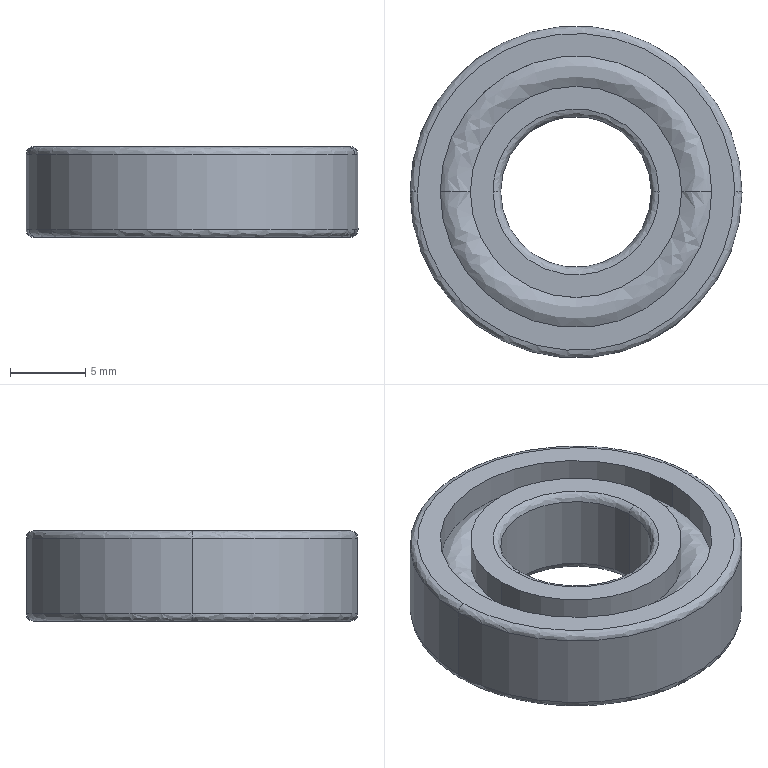Part | SolidWorks | features BaseBody 1 | 1 solid | 28 faces | box 22 x 22 x 6 mm | volume 1473 mm3 | spline 12 | cylinder 12 | plane 4 | commonest cylinder face diameters 14 x4 18 x4 10 x2 22 x2
STEP:
#1=CARTESIAN_POINT('',(11.,0.,2.5));
#2=VERTEX_POINT('',#1);
#3=CARTESIAN_POINT('',(-11.,0.,2.5));
#4=VERTEX_POINT('',#3);
#5=CARTESIAN_POINT('',(0.,0.,2.5));
#6=DIRECTION('',(0.,0.,-1.));
#7=DIRECTION('',(1.,0.,0.));
#8=AXIS2_PLACEMENT_3D('',#5,#6,#7);
#9=CIRCLE('',#8,11.);
#10=EDGE_CURVE('',#2,#4,#9,.T.);
#11=ORIENTED_EDGE('',*,*,#10,.F.);
#12=CARTESIAN_POINT('',(10.5,0.,3.));
#13=VERTEX_POINT('',#12);
#14=CARTESIAN_POINT('',(10.5,0.,2.5));
#15=DIRECTION('',(0.,-1.,0.));
#16=DIRECTION('',(1.,0.,0.));
#17=AXIS2_PLACEMENT_3D('',#14,#15,#16);
#18=CIRCLE('',#17,0.5);
#19=EDGE_CURVE('',#2,#13,#18,.T.);
#20=ORIENTED_EDGE('',*,*,#19,.T.);
#21=CARTESIAN_POINT('',(-10.5,0.,3.));
#22=VERTEX_POINT('',#21);
#23=CARTESIAN_POINT('',(10.5,0.,3.));
#24=CARTESIAN_POINT('',(10.5,-21.,3.));
#25=CARTESIAN_POINT('',(-10.5,-21.,3.));
#26=CARTESIAN_POINT('',(-10.5,0.,3.));
#27=(BOUNDED_CURVE()B_SPLINE_CURVE(3,(#23,#24,#25,#26),.UNSPECIFIED.,.F.,.T.)B_SPLINE_CURVE_WITH_KNOTS((4,4),(0.,1.),.UNSPECIFIED.)CURVE()GEOMETRIC_REPRESENTATION_ITEM()RATIONAL_B_SPLINE_CURVE((1.,0.3333,0.3333,1.))REPRESENTATION_ITEM(''));
#28=EDGE_CURVE('',#13,#22,#27,.T.);
#29=ORIENTED_EDGE('',*,*,#28,.T.);
#30=CARTESIAN_POINT('',(-10.5,0.,2.5));
#31=DIRECTION('',(0.,1.,0.));
#32=DIRECTION('',(-1.,0.,0.));
#33=AXIS2_PLACEMENT_3D('',#30,#31,#32);
#34=CIRCLE('',#33,0.5);
#35=EDGE_CURVE('',#4,#22,#34,.T.);
#36=ORIENTED_EDGE('',*,*,#35,.F.);
#37=EDGE_LOOP('',(#11,#20,#29,#36));
#38=FACE_OUTER_BOUND('',#37,.T.);
#39=CARTESIAN_POINT('',(11.,0.,2.5));
#40=CARTESIAN_POINT('',(11.,-22.,2.5));
#41=CARTESIAN_POINT('',(-11.,-22.,2.5));
#42=CARTESIAN_POINT('',(-11.,0.,2.5));
#43=CARTESIAN_POINT('',(11.,0.,2.793));
#44=CARTESIAN_POINT('',(11.,-22.,2.793));
#45=CARTESIAN_POINT('',(-11.,-22.,2.793));
#46=CARTESIAN_POINT('',(-11.,0.,2.793));
#47=CARTESIAN_POINT('',(10.793,0.,3.));
#48=CARTESIAN_POINT('',(10.793,-21.586,3.));
#49=CARTESIAN_POINT('',(-10.793,-21.586,3.));
#50=CARTESIAN_POINT('',(-10.793,0.,3.));
#51=CARTESIAN_POINT('',(10.5,0.,3.));
#52=CARTESIAN_POINT('',(10.5,-21.,3.));
#53=CARTESIAN_POINT('',(-10.5,-21.,3.));
#54=CARTESIAN_POINT('',(-10.5,0.,3.));
#55=(BOUNDED_SURFACE()B_SPLINE_SURFACE(3,3,((#39,#40,#41,#42),(#43,#44,#45,#46),(#47,#48,#49,#50),(#51,#52,#53,#54)),.UNSPECIFIED.,.F.,.F.,.T.)B_SPLINE_SURFACE_WITH_KNOTS((4,4),(4,4),(0.,1.),(0.,1.),.UNSPECIFIED.)GEOMETRIC_REPRESENTATION_ITEM()RATIONAL_B_SPLINE_SURFACE(((1.,0.3333,0.3333,1.),(0.8047,0.2682,0.2682,0.8047),(0.8047,0.2682,0.2682,0.8047),(1.,0.3333,0.3333,1.)))REPRESENTATION_ITEM('')SURFACE());
#56=ADVANCED_FACE('',(#38),#55,.T.);
#57=CARTESIAN_POINT('',(-11.,0.,-2.5));
#58=VERTEX_POINT('',#57);
#59=CARTESIAN_POINT('',(11.,0.,-2.5));
#60=VERTEX_POINT('',#59);
#61=CARTESIAN_POINT('',(0.,0.,-2.5));
#62=DIRECTION('',(0.,0.,1.));
#63=DIRECTION('',(1.,0.,0.));
#64=AXIS2_PLACEMENT_3D('',#61,#62,#63);
#65=CIRCLE('',#64,11.);
#66=EDGE_CURVE('',#58,#60,#65,.T.);
#67=ORIENTED_EDGE('',*,*,#66,.F.);
#68=CARTESIAN_POINT('',(-10.5,0.,-3.));
#69=VERTEX_POINT('',#68);
#70=CARTESIAN_POINT('',(-10.5,0.,-2.5));
#71=DIRECTION('',(0.,-1.,0.));
#72=DIRECTION('',(-1.,0.,0.));
#73=AXIS2_PLACEMENT_3D('',#70,#71,#72);
#74=CIRCLE('',#73,0.5);
#75=EDGE_CURVE('',#58,#69,#74,.T.);
#76=ORIENTED_EDGE('',*,*,#75,.T.);
#77=CARTESIAN_POINT('',(10.5,0.,-3.));
#78=VERTEX_POINT('',#77);
#79=CARTESIAN_POINT('',(-10.5,0.,-3.));
#80=CARTESIAN_POINT('',(-10.5,-21.,-3.));
#81=CARTESIAN_POINT('',(10.5,-21.,-3.));
#82=CARTESIAN_POINT('',(10.5,0.,-3.));
#83=(BOUNDED_CURVE()B_SPLINE_CURVE(3,(#79,#80,#81,#82),.UNSPECIFIED.,.F.,.T.)B_SPLINE_CURVE_WITH_KNOTS((4,4),(0.,1.),.UNSPECIFIED.)CURVE()GEOMETRIC_REPRESENTATION_ITEM()RATIONAL_B_SPLINE_CURVE((1.,0.3333,0.3333,1.))REPRESENTATION_ITEM(''));
#84=EDGE_CURVE('',#69,#78,#83,.T.);
#85=ORIENTED_EDGE('',*,*,#84,.T.);
#86=CARTESIAN_POINT('',(10.5,0.,-2.5));
#87=DIRECTION('',(0.,1.,0.));
#88=DIRECTION('',(1.,0.,0.));
#89=AXIS2_PLACEMENT_3D('',#86,#87,#88);
#90=CIRCLE('',#89,0.5);
#91=EDGE_CURVE('',#60,#78,#90,.T.);
#92=ORIENTED_EDGE('',*,*,#91,.F.);
#93=EDGE_LOOP('',(#67,#76,#85,#92));
#94=FACE_OUTER_BOUND('',#93,.T.);
#95=CARTESIAN_POINT('',(-11.,0.,-2.5));
#96=CARTESIAN_POINT('',(-11.,-22.,-2.5));
#97=CARTESIAN_POINT('',(11.,-22.,-2.5));
#98=CARTESIAN_POINT('',(11.,0.,-2.5));
#99=CARTESIAN_POINT('',(-11.,0.,-2.793));
#100=CARTESIAN_POINT('',(-11.,-22.,-2.793));
#101=CARTESIAN_POINT('',(11.,-22.,-2.793));
#102=CARTESIAN_POINT('',(11.,0.,-2.793));
#103=CARTESIAN_POINT('',(-10.793,0.,-3.));
#104=CARTESIAN_POINT('',(-10.793,-21.586,-3.));
#105=CARTESIAN_POINT('',(10.793,-21.586,-3.));
#106=CARTESIAN_POINT('',(10.793,0.,-3.));
#107=CARTESIAN_POINT('',(-10.5,0.,-3.));
#108=CARTESIAN_POINT('',(-10.5,-21.,-3.));
#109=CARTESIAN_POINT('',(10.5,-21.,-3.));
#110=CARTESIAN_POINT('',(10.5,0.,-3.));
#111=(BOUNDED_SURFACE()B_SPLINE_SURFACE(3,3,((#95,#96,#97,#98),(#99,#100,#101,#102),(#103,#104,#105,#106),(#107,#108,#109,#110)),.UNSPECIFIED.,.F.,.F.,.T.)B_SPLINE_SURFACE_WITH_KNOTS((4,4),(4,4),(0.,1.),(0.,1.),.UNSPECIFIED.)GEOMETRIC_REPRESENTATION_ITEM()RATIONAL_B_SPLINE_SURFACE(((1.,0.3333,0.3333,1.),(0.8047,0.2682,0.2682,0.8047),(0.8047,0.2682,0.2682,0.8047),(1.,0.3333,0.3333,1.)))REPRESENTATION_ITEM('')SURFACE());
#112=ADVANCED_FACE('',(#94),#111,.T.);
#113=CARTESIAN_POINT('',(-9.,0.,1.118));
#114=VERTEX_POINT('',#113);
#115=CARTESIAN_POINT('',(9.,0.,1.118));
#116=VERTEX_POINT('',#115);
#117=CARTESIAN_POINT('',(0.,0.,1.118));
#118=DIRECTION('',(0.,0.,1.));
#119=DIRECTION('',(1.,0.,0.));
#120=AXIS2_PLACEMENT_3D('',#117,#118,#119);
#121=CIRCLE('',#120,9.);
#122=EDGE_CURVE('',#114,#116,#121,.T.);
#123=ORIENTED_EDGE('',*,*,#122,.T.);
#124=CARTESIAN_POINT('',(7.,0.,1.118));
#125=VERTEX_POINT('',#124);
#126=CARTESIAN_POINT('',(8.,0.,0.));
#127=DIRECTION('',(0.,-1.,0.));
#128=DIRECTION('',(1.,0.,0.));
#129=AXIS2_PLACEMENT_3D('',#126,#127,#128);
#130=CIRCLE('',#129,1.5);
#131=EDGE_CURVE('',#116,#125,#130,.T.);
#132=ORIENTED_EDGE('',*,*,#131,.T.);
#133=CARTESIAN_POINT('',(-7.,0.,1.118));
#134=VERTEX_POINT('',#133);
#135=CARTESIAN_POINT('',(0.,0.,1.118));
#136=DIRECTION('',(0.,0.,-1.));
#137=DIRECTION('',(-1.,0.,0.));
#138=AXIS2_PLACEMENT_3D('',#135,#136,#137);
#139=CIRCLE('',#138,7.);
#140=EDGE_CURVE('',#125,#134,#139,.T.);
#141=ORIENTED_EDGE('',*,*,#140,.T.);
#142=CARTESIAN_POINT('',(-8.,0.,0.));
#143=DIRECTION('',(0.,1.,0.));
#144=DIRECTION('',(-1.,0.,0.));
#145=AXIS2_PLACEMENT_3D('',#142,#143,#144);
#146=CIRCLE('',#145,1.5);
#147=EDGE_CURVE('',#114,#134,#146,.T.);
#148=ORIENTED_EDGE('',*,*,#147,.F.);
#149=EDGE_LOOP('',(#123,#132,#141,#148));
#150=FACE_OUTER_BOUND('',#149,.T.);
#151=CARTESIAN_POINT('',(9.,0.,1.118));
#152=CARTESIAN_POINT('',(9.,-18.,1.118));
#153=CARTESIAN_POINT('',(-9.,-18.,1.118));
#154=CARTESIAN_POINT('',(-9.,0.,1.118));
#155=CARTESIAN_POINT('',(8.401,0.,1.653));
#156=CARTESIAN_POINT('',(8.401,-16.803,1.653));
#157=CARTESIAN_POINT('',(-8.401,-16.803,1.653));
#158=CARTESIAN_POINT('',(-8.401,0.,1.653));
#159=CARTESIAN_POINT('',(7.599,0.,1.653));
#160=CARTESIAN_POINT('',(7.599,-15.197,1.653));
#161=CARTESIAN_POINT('',(-7.599,-15.197,1.653));
#162=CARTESIAN_POINT('',(-7.599,0.,1.653));
#163=CARTESIAN_POINT('',(7.,0.,1.118));
#164=CARTESIAN_POINT('',(7.,-14.,1.118));
#165=CARTESIAN_POINT('',(-7.,-14.,1.118));
#166=CARTESIAN_POINT('',(-7.,0.,1.118));
#167=(BOUNDED_SURFACE()B_SPLINE_SURFACE(3,3,((#151,#152,#153,#154),(#155,#156,#157,#158),(#159,#160,#161,#162),(#163,#164,#165,#166)),.UNSPECIFIED.,.F.,.F.,.T.)B_SPLINE_SURFACE_WITH_KNOTS((4,4),(4,4),(0.,1.),(0.,1.),.UNSPECIFIED.)GEOMETRIC_REPRESENTATION_ITEM()RATIONAL_B_SPLINE_SURFACE(((1.,0.3333,0.3333,1.),(0.8302,0.2767,0.2767,0.8302),(0.8302,0.2767,0.2767,0.8302),(1.,0.3333,0.3333,1.)))REPRESENTATION_ITEM('')SURFACE());
#168=ADVANCED_FACE('',(#150),#167,.T.);
#169=CARTESIAN_POINT('',(-7.,0.,-1.118));
#170=VERTEX_POINT('',#169);
#171=CARTESIAN_POINT('',(7.,0.,-1.118));
#172=VERTEX_POINT('',#171);
#173=CARTESIAN_POINT('',(0.,0.,-1.118));
#174=DIRECTION('',(0.,0.,1.));
#175=DIRECTION('',(-1.,0.,0.));
#176=AXIS2_PLACEMENT_3D('',#173,#174,#175);
#177=CIRCLE('',#176,7.);
#178=EDGE_CURVE('',#170,#172,#177,.T.);
#179=ORIENTED_EDGE('',*,*,#178,.T.);
#180=CARTESIAN_POINT('',(9.,0.,-1.118));
#181=VERTEX_POINT('',#180);
#182=CARTESIAN_POINT('',(8.,0.,0.));
#183=DIRECTION('',(0.,-1.,0.));
#184=DIRECTION('',(1.,0.,0.));
#185=AXIS2_PLACEMENT_3D('',#182,#183,#184);
#186=CIRCLE('',#185,1.5);
#187=EDGE_CURVE('',#172,#181,#186,.T.);
#188=ORIENTED_EDGE('',*,*,#187,.T.);
#189=CARTESIAN_POINT('',(-9.,0.,-1.118));
#190=VERTEX_POINT('',#189);
#191=CARTESIAN_POINT('',(0.,0.,-1.118));
#192=DIRECTION('',(0.,0.,-1.));
#193=DIRECTION('',(1.,0.,0.));
#194=AXIS2_PLACEMENT_3D('',#191,#192,#193);
#195=CIRCLE('',#194,9.);
#196=EDGE_CURVE('',#181,#190,#195,.T.);
#197=ORIENTED_EDGE('',*,*,#196,.T.);
#198=CARTESIAN_POINT('',(-8.,0.,0.));
#199=DIRECTION('',(0.,1.,0.));
#200=DIRECTION('',(-1.,0.,0.));
#201=AXIS2_PLACEMENT_3D('',#198,#199,#200);
#202=CIRCLE('',#201,1.5);
#203=EDGE_CURVE('',#170,#190,#202,.T.);
#204=ORIENTED_EDGE('',*,*,#203,.F.);
#205=EDGE_LOOP('',(#179,#188,#197,#204));
#206=FACE_OUTER_BOUND('',#205,.T.);
#207=CARTESIAN_POINT('',(7.,0.,-1.118));
#208=CARTESIAN_POINT('',(7.,-14.,-1.118));
#209=CARTESIAN_POINT('',(-7.,-14.,-1.118));
#210=CARTESIAN_POINT('',(-7.,0.,-1.118));
#211=CARTESIAN_POINT('',(7.599,0.,-1.653));
#212=CARTESIAN_POINT('',(7.599,-15.197,-1.653));
#213=CARTESIAN_POINT('',(-7.599,-15.197,-1.653));
#214=CARTESIAN_POINT('',(-7.599,0.,-1.653));
#215=CARTESIAN_POINT('',(8.401,0.,-1.653));
#216=CARTESIAN_POINT('',(8.401,-16.803,-1.653));
#217=CARTESIAN_POINT('',(-8.401,-16.803,-1.653));
#218=CARTESIAN_POINT('',(-8.401,0.,-1.653));
#219=CARTESIAN_POINT('',(9.,0.,-1.118));
#220=CARTESIAN_POINT('',(9.,-18.,-1.118));
#221=CARTESIAN_POINT('',(-9.,-18.,-1.118));
#222=CARTESIAN_POINT('',(-9.,0.,-1.118));
#223=(BOUNDED_SURFACE()B_SPLINE_SURFACE(3,3,((#207,#208,#209,#210),(#211,#212,#213,#214),(#215,#216,#217,#218),(#219,#220,#221,#222)),.UNSPECIFIED.,.F.,.F.,.T.)B_SPLINE_SURFACE_WITH_KNOTS((4,4),(4,4),(0.,1.),(0.,1.),.UNSPECIFIED.)GEOMETRIC_REPRESENTATION_ITEM()RATIONAL_B_SPLINE_SURFACE(((1.,0.3333,0.3333,1.),(0.8302,0.2767,0.2767,0.8302),(0.8302,0.2767,0.2767,0.8302),(1.,0.3333,0.3333,1.)))REPRESENTATION_ITEM('')SURFACE());
#224=ADVANCED_FACE('',(#206),#223,.T.);
#225=CARTESIAN_POINT('',(-5.5,0.,3.));
#226=VERTEX_POINT('',#225);
#227=CARTESIAN_POINT('',(5.5,0.,3.));
#228=VERTEX_POINT('',#227);
#229=CARTESIAN_POINT('',(-5.5,0.,3.));
#230=CARTESIAN_POINT('',(-5.5,-11.,3.));
#231=CARTESIAN_POINT('',(5.5,-11.,3.));
#232=CARTESIAN_POINT('',(5.5,0.,3.));
#233=(BOUNDED_CURVE()B_SPLINE_CURVE(3,(#229,#230,#231,#232),.UNSPECIFIED.,.F.,.F.)B_SPLINE_CURVE_WITH_KNOTS((4,4),(0.,1.),.UNSPECIFIED.)CURVE()GEOMETRIC_REPRESENTATION_ITEM()RATIONAL_B_SPLINE_CURVE((1.,0.3333,0.3333,1.))REPRESENTATION_ITEM(''));
#234=EDGE_CURVE('',#226,#228,#233,.T.);
#235=ORIENTED_EDGE('',*,*,#234,.T.);
#236=CARTESIAN_POINT('',(5.,0.,2.5));
#237=VERTEX_POINT('',#236);
#238=CARTESIAN_POINT('',(5.5,0.,2.5));
#239=DIRECTION('',(0.,-1.,0.));
#240=DIRECTION('',(1.,0.,0.));
#241=AXIS2_PLACEMENT_3D('',#238,#239,#240);
#242=CIRCLE('',#241,0.5);
#243=EDGE_CURVE('',#228,#237,#242,.T.);
#244=ORIENTED_EDGE('',*,*,#243,.T.);
#245=CARTESIAN_POINT('',(-5.,0.,2.5));
#246=VERTEX_POINT('',#245);
#247=CARTESIAN_POINT('',(0.,0.,2.5));
#248=DIRECTION('',(0.,0.,-1.));
#249=DIRECTION('',(-1.,0.,0.));
#250=AXIS2_PLACEMENT_3D('',#247,#248,#249);
#251=CIRCLE('',#250,5.);
#252=EDGE_CURVE('',#237,#246,#251,.T.);
#253=ORIENTED_EDGE('',*,*,#252,.T.);
#254=CARTESIAN_POINT('',(-5.5,0.,2.5));
#255=DIRECTION('',(0.,1.,0.));
#256=DIRECTION('',(-1.,0.,0.));
#257=AXIS2_PLACEMENT_3D('',#254,#255,#256);
#258=CIRCLE('',#257,0.5);
#259=EDGE_CURVE('',#226,#246,#258,.T.);
#260=ORIENTED_EDGE('',*,*,#259,.F.);
#261=EDGE_LOOP('',(#235,#244,#253,#260));
#262=FACE_OUTER_BOUND('',#261,.T.);
#263=CARTESIAN_POINT('',(5.5,0.,3.));
#264=CARTESIAN_POINT('',(5.5,-11.,3.));
#265=CARTESIAN_POINT('',(-5.5,-11.,3.));
#266=CARTESIAN_POINT('',(-5.5,0.,3.));
#267=CARTESIAN_POINT('',(5.207,0.,3.));
#268=CARTESIAN_POINT('',(5.207,-10.414,3.));
#269=CARTESIAN_POINT('',(-5.207,-10.414,3.));
#270=CARTESIAN_POINT('',(-5.207,0.,3.));
#271=CARTESIAN_POINT('',(5.,0.,2.793));
#272=CARTESIAN_POINT('',(5.,-10.,2.793));
#273=CARTESIAN_POINT('',(-5.,-10.,2.793));
#274=CARTESIAN_POINT('',(-5.,0.,2.793));
#275=CARTESIAN_POINT('',(5.,0.,2.5));
#276=CARTESIAN_POINT('',(5.,-10.,2.5));
#277=CARTESIAN_POINT('',(-5.,-10.,2.5));
#278=CARTESIAN_POINT('',(-5.,0.,2.5));
#279=(BOUNDED_SURFACE()B_SPLINE_SURFACE(3,3,((#263,#264,#265,#266),(#267,#268,#269,#270),(#271,#272,#273,#274),(#275,#276,#277,#278)),.UNSPECIFIED.,.F.,.F.,.T.)B_SPLINE_SURFACE_WITH_KNOTS((4,4),(4,4),(0.,1.),(0.,1.),.UNSPECIFIED.)GEOMETRIC_REPRESENTATION_ITEM()RATIONAL_B_SPLINE_SURFACE(((1.,0.3333,0.3333,1.),(0.8047,0.2682,0.2682,0.8047),(0.8047,0.2682,0.2682,0.8047),(1.,0.3333,0.3333,1.)))REPRESENTATION_ITEM('')SURFACE());
#280=ADVANCED_FACE('',(#262),#279,.T.);
#281=CARTESIAN_POINT('',(5.5,0.,-3.));
#282=VERTEX_POINT('',#281);
#283=CARTESIAN_POINT('',(-5.5,0.,-3.));
#284=VERTEX_POINT('',#283);
#285=CARTESIAN_POINT('',(5.5,0.,-3.));
#286=CARTESIAN_POINT('',(5.5,-11.,-3.));
#287=CARTESIAN_POINT('',(-5.5,-11.,-3.));
#288=CARTESIAN_POINT('',(-5.5,0.,-3.));
#289=(BOUNDED_CURVE()B_SPLINE_CURVE(3,(#285,#286,#287,#288),.UNSPECIFIED.,.F.,.F.)B_SPLINE_CURVE_WITH_KNOTS((4,4),(0.,1.),.UNSPECIFIED.)CURVE()GEOMETRIC_REPRESENTATION_ITEM()RATIONAL_B_SPLINE_CURVE((1.,0.3333,0.3333,1.))REPRESENTATION_ITEM(''));
#290=EDGE_CURVE('',#282,#284,#289,.T.);
#291=ORIENTED_EDGE('',*,*,#290,.T.);
#292=CARTESIAN_POINT('',(-5.,0.,-2.5));
#293=VERTEX_POINT('',#292);
#294=CARTESIAN_POINT('',(-5.5,0.,-2.5));
#295=DIRECTION('',(0.,-1.,0.));
#296=DIRECTION('',(-1.,0.,0.));
#297=AXIS2_PLACEMENT_3D('',#294,#295,#296);
#298=CIRCLE('',#297,0.5);
#299=EDGE_CURVE('',#284,#293,#298,.T.);
#300=ORIENTED_EDGE('',*,*,#299,.T.);
#301=CARTESIAN_POINT('',(5.,0.,-2.5));
#302=VERTEX_POINT('',#301);
#303=CARTESIAN_POINT('',(0.,0.,-2.5));
#304=DIRECTION('',(0.,0.,1.));
#305=DIRECTION('',(1.,0.,0.));
#306=AXIS2_PLACEMENT_3D('',#303,#304,#305);
#307=CIRCLE('',#306,5.);
#308=EDGE_CURVE('',#293,#302,#307,.T.);
#309=ORIENTED_EDGE('',*,*,#308,.T.);
#310=CARTESIAN_POINT('',(5.5,0.,-2.5));
#311=DIRECTION('',(0.,1.,0.));
#312=DIRECTION('',(1.,0.,0.));
#313=AXIS2_PLACEMENT_3D('',#310,#311,#312);
#314=CIRCLE('',#313,0.5);
#315=EDGE_CURVE('',#282,#302,#314,.T.);
#316=ORIENTED_EDGE('',*,*,#315,.F.);
#317=EDGE_LOOP('',(#291,#300,#309,#316));
#318=FACE_OUTER_BOUND('',#317,.T.);
#319=CARTESIAN_POINT('',(-5.5,0.,-3.));
#320=CARTESIAN_POINT('',(-5.5,-11.,-3.));
#321=CARTESIAN_POINT('',(5.5,-11.,-3.));
#322=CARTESIAN_POINT('',(5.5,0.,-3.));
#323=CARTESIAN_POINT('',(-5.207,0.,-3.));
#324=CARTESIAN_POINT('',(-5.207,-10.414,-3.));
#325=CARTESIAN_POINT('',(5.207,-10.414,-3.));
#326=CARTESIAN_POINT('',(5.207,0.,-3.));
#327=CARTESIAN_POINT('',(-5.,0.,-2.793));
#328=CARTESIAN_POINT('',(-5.,-10.,-2.793));
#329=CARTESIAN_POINT('',(5.,-10.,-2.793));
#330=CARTESIAN_POINT('',(5.,0.,-2.793));
#331=CARTESIAN_POINT('',(-5.,0.,-2.5));
#332=CARTESIAN_POINT('',(-5.,-10.,-2.5));
#333=CARTESIAN_POINT('',(5.,-10.,-2.5));
#334=CARTESIAN_POINT('',(5.,0.,-2.5));
#335=(BOUNDED_SURFACE()B_SPLINE_SURFACE(3,3,((#319,#320,#321,#322),(#323,#324,#325,#326),(#327,#328,#329,#330),(#331,#332,#333,#334)),.UNSPECIFIED.,.F.,.F.,.T.)B_SPLINE_SURFACE_WITH_KNOTS((4,4),(4,4),(0.,1.),(0.,1.),.UNSPECIFIED.)GEOMETRIC_REPRESENTATION_ITEM()RATIONAL_B_SPLINE_SURFACE(((1.,0.3333,0.3333,1.),(0.8047,0.2682,0.2682,0.8047),(0.8047,0.2682,0.2682,0.8047),(1.,0.3333,0.3333,1.)))REPRESENTATION_ITEM('')SURFACE());
#336=ADVANCED_FACE('',(#318),#335,.T.);
#337=CARTESIAN_POINT('',(0.,0.,-2.5));
#338=DIRECTION('',(0.,0.,1.));
#339=DIRECTION('',(1.,0.,0.));
#340=AXIS2_PLACEMENT_3D('',#337,#338,#339);
#341=CIRCLE('',#340,11.);
#342=EDGE_CURVE('',#60,#58,#341,.T.);
#343=ORIENTED_EDGE('',*,*,#342,.T.);
#344=CARTESIAN_POINT('',(-11.,0.,50.392));
#345=DIRECTION('',(0.,0.,1.));
#346=VECTOR('',#345,1000.);
#347=LINE('',#344,#346);
#348=EDGE_CURVE('',#58,#4,#347,.T.);
#349=ORIENTED_EDGE('',*,*,#348,.T.);
#350=CARTESIAN_POINT('',(0.,0.,2.5));
#351=DIRECTION('',(0.,0.,-1.));
#352=DIRECTION('',(1.,0.,0.));
#353=AXIS2_PLACEMENT_3D('',#350,#351,#352);
#354=CIRCLE('',#353,11.);
#355=EDGE_CURVE('',#4,#2,#354,.T.);
#356=ORIENTED_EDGE('',*,*,#355,.T.);
#357=CARTESIAN_POINT('',(11.,0.,50.392));
#358=DIRECTION('',(0.,0.,1.));
#359=VECTOR('',#358,1000.);
#360=LINE('',#357,#359);
#361=EDGE_CURVE('',#60,#2,#360,.T.);
#362=ORIENTED_EDGE('',*,*,#361,.F.);
#363=EDGE_LOOP('',(#343,#349,#356,#362));
#364=FACE_OUTER_BOUND('',#363,.T.);
#365=CARTESIAN_POINT('',(0.,0.,50.392));
#366=DIRECTION('',(0.,0.,1.));
#367=DIRECTION('',(1.,0.,0.));
#368=AXIS2_PLACEMENT_3D('',#365,#366,#367);
#369=CYLINDRICAL_SURFACE('',#368,11.);
#370=ADVANCED_FACE('',(#364),#369,.T.);
#371=ORIENTED_EDGE('',*,*,#122,.F.);
#372=CARTESIAN_POINT('',(-9.,0.,3.));
#373=VERTEX_POINT('',#372);
#374=CARTESIAN_POINT('',(-9.,0.,50.392));
#375=DIRECTION('',(0.,0.,1.));
#376=VECTOR('',#375,1000.);
#377=LINE('',#374,#376);
#378=EDGE_CURVE('',#114,#373,#377,.T.);
#379=ORIENTED_EDGE('',*,*,#378,.T.);
#380=CARTESIAN_POINT('',(9.,0.,3.));
#381=VERTEX_POINT('',#380);
#382=CARTESIAN_POINT('',(0.,0.,3.));
#383=DIRECTION('',(0.,0.,1.));
#384=DIRECTION('',(1.,0.,0.));
#385=AXIS2_PLACEMENT_3D('',#382,#383,#384);
#386=CIRCLE('',#385,9.);
#387=EDGE_CURVE('',#373,#381,#386,.T.);
#388=ORIENTED_EDGE('',*,*,#387,.T.);
#389=CARTESIAN_POINT('',(9.,0.,50.392));
#390=DIRECTION('',(0.,0.,1.));
#391=VECTOR('',#390,1000.);
#392=LINE('',#389,#391);
#393=EDGE_CURVE('',#116,#381,#392,.T.);
#394=ORIENTED_EDGE('',*,*,#393,.F.);
#395=EDGE_LOOP('',(#371,#379,#388,#394));
#396=FACE_OUTER_BOUND('',#395,.T.);
#397=CARTESIAN_POINT('',(0.,0.,50.392));
#398=DIRECTION('',(0.,0.,1.));
#399=DIRECTION('',(1.,0.,0.));
#400=AXIS2_PLACEMENT_3D('',#397,#398,#399);
#401=CYLINDRICAL_SURFACE('',#400,9.);
#402=ADVANCED_FACE('',(#396),#401,.F.);
#403=CARTESIAN_POINT('',(9.,0.,-3.));
#404=VERTEX_POINT('',#403);
#405=CARTESIAN_POINT('',(-9.,0.,-3.));
#406=VERTEX_POINT('',#405);
#407=CARTESIAN_POINT('',(0.,0.,-3.));
#408=DIRECTION('',(0.,0.,-1.));
#409=DIRECTION('',(1.,0.,0.));
#410=AXIS2_PLACEMENT_3D('',#407,#408,#409);
#411=CIRCLE('',#410,9.);
#412=EDGE_CURVE('',#404,#406,#411,.T.);
#413=ORIENTED_EDGE('',*,*,#412,.T.);
#414=CARTESIAN_POINT('',(-9.,0.,50.392));
#415=DIRECTION('',(0.,0.,1.));
#416=VECTOR('',#415,1000.);
#417=LINE('',#414,#416);
#418=EDGE_CURVE('',#406,#190,#417,.T.);
#419=ORIENTED_EDGE('',*,*,#418,.T.);
#420=ORIENTED_EDGE('',*,*,#196,.F.);
#421=CARTESIAN_POINT('',(9.,0.,50.392));
#422=DIRECTION('',(0.,0.,1.));
#423=VECTOR('',#422,1000.);
#424=LINE('',#421,#423);
#425=EDGE_CURVE('',#404,#181,#424,.T.);
#426=ORIENTED_EDGE('',*,*,#425,.F.);
#427=EDGE_LOOP('',(#413,#419,#420,#426));
#428=FACE_OUTER_BOUND('',#427,.T.);
#429=CARTESIAN_POINT('',(0.,0.,50.392));
#430=DIRECTION('',(0.,0.,1.));
#431=DIRECTION('',(1.,0.,0.));
#432=AXIS2_PLACEMENT_3D('',#429,#430,#431);
#433=CYLINDRICAL_SURFACE('',#432,9.);
#434=ADVANCED_FACE('',(#428),#433,.F.);
#435=CARTESIAN_POINT('',(0.,0.,1.118));
#436=DIRECTION('',(0.,0.,-1.));
#437=DIRECTION('',(-1.,0.,0.));
#438=AXIS2_PLACEMENT_3D('',#435,#436,#437);
#439=CIRCLE('',#438,7.);
#440=EDGE_CURVE('',#134,#125,#439,.T.);
#441=ORIENTED_EDGE('',*,*,#440,.F.);
#442=CARTESIAN_POINT('',(-7.,0.,3.));
#443=VERTEX_POINT('',#442);
#444=CARTESIAN_POINT('',(-7.,0.,70.863));
#445=DIRECTION('',(0.,0.,1.));
#446=VECTOR('',#445,1000.);
#447=LINE('',#444,#446);
#448=EDGE_CURVE('',#134,#443,#447,.T.);
#449=ORIENTED_EDGE('',*,*,#448,.T.);
#450=CARTESIAN_POINT('',(7.,0.,3.));
#451=VERTEX_POINT('',#450);
#452=CARTESIAN_POINT('',(0.,0.,3.));
#453=DIRECTION('',(0.,0.,-1.));
#454=DIRECTION('',(1.,0.,0.));
#455=AXIS2_PLACEMENT_3D('',#452,#453,#454);
#456=CIRCLE('',#455,7.);
#457=EDGE_CURVE('',#443,#451,#456,.T.);
#458=ORIENTED_EDGE('',*,*,#457,.T.);
#459=CARTESIAN_POINT('',(7.,0.,70.863));
#460=DIRECTION('',(0.,0.,1.));
#461=VECTOR('',#460,1000.);
#462=LINE('',#459,#461);
#463=EDGE_CURVE('',#125,#451,#462,.T.);
#464=ORIENTED_EDGE('',*,*,#463,.F.);
#465=EDGE_LOOP('',(#441,#449,#458,#464));
#466=FACE_OUTER_BOUND('',#465,.T.);
#467=CARTESIAN_POINT('',(0.,0.,70.863));
#468=DIRECTION('',(0.,0.,1.));
#469=DIRECTION('',(1.,0.,0.));
#470=AXIS2_PLACEMENT_3D('',#467,#468,#469);
#471=CYLINDRICAL_SURFACE('',#470,7.);
#472=ADVANCED_FACE('',(#466),#471,.T.);
#473=CARTESIAN_POINT('',(7.,0.,-3.));
#474=VERTEX_POINT('',#473);
#475=CARTESIAN_POINT('',(-7.,0.,-3.));
#476=VERTEX_POINT('',#475);
#477=CARTESIAN_POINT('',(0.,0.,-3.));
#478=DIRECTION('',(0.,0.,1.));
#479=DIRECTION('',(1.,0.,0.));
#480=AXIS2_PLACEMENT_3D('',#477,#478,#479);
#481=CIRCLE('',#480,7.);
#482=EDGE_CURVE('',#474,#476,#481,.T.);
#483=ORIENTED_EDGE('',*,*,#482,.T.);
#484=CARTESIAN_POINT('',(-7.,0.,70.863));
#485=DIRECTION('',(0.,0.,1.));
#486=VECTOR('',#485,1000.);
#487=LINE('',#484,#486);
#488=EDGE_CURVE('',#476,#170,#487,.T.);
#489=ORIENTED_EDGE('',*,*,#488,.T.);
#490=CARTESIAN_POINT('',(0.,0.,-1.118));
#491=DIRECTION('',(0.,0.,1.));
#492=DIRECTION('',(-1.,0.,0.));
#493=AXIS2_PLACEMENT_3D('',#490,#491,#492);
#494=CIRCLE('',#493,7.);
#495=EDGE_CURVE('',#172,#170,#494,.T.);
#496=ORIENTED_EDGE('',*,*,#495,.F.);
#497=CARTESIAN_POINT('',(7.,0.,70.863));
#498=DIRECTION('',(0.,0.,1.));
#499=VECTOR('',#498,1000.);
#500=LINE('',#497,#499);
#501=EDGE_CURVE('',#474,#172,#500,.T.);
#502=ORIENTED_EDGE('',*,*,#501,.F.);
#503=EDGE_LOOP('',(#483,#489,#496,#502));
#504=FACE_OUTER_BOUND('',#503,.T.);
#505=CARTESIAN_POINT('',(0.,0.,70.863));
#506=DIRECTION('',(0.,0.,1.));
#507=DIRECTION('',(1.,0.,0.));
#508=AXIS2_PLACEMENT_3D('',#505,#506,#507);
#509=CYLINDRICAL_SURFACE('',#508,7.);
#510=ADVANCED_FACE('',(#504),#509,.T.);
#511=ORIENTED_EDGE('',*,*,#308,.F.);
#512=CARTESIAN_POINT('',(-5.,0.,70.863));
#513=DIRECTION('',(0.,0.,1.));
#514=VECTOR('',#513,1000.);
#515=LINE('',#512,#514);
#516=EDGE_CURVE('',#293,#246,#515,.T.);
#517=ORIENTED_EDGE('',*,*,#516,.T.);
#518=ORIENTED_EDGE('',*,*,#252,.F.);
#519=CARTESIAN_POINT('',(5.,0.,70.863));
#520=DIRECTION('',(0.,0.,1.));
#521=VECTOR('',#520,1000.);
#522=LINE('',#519,#521);
#523=EDGE_CURVE('',#302,#237,#522,.T.);
#524=ORIENTED_EDGE('',*,*,#523,.F.);
#525=EDGE_LOOP('',(#511,#517,#518,#524));
#526=FACE_OUTER_BOUND('',#525,.T.);
#527=CARTESIAN_POINT('',(0.,0.,70.863));
#528=DIRECTION('',(0.,0.,1.));
#529=DIRECTION('',(1.,0.,0.));
#530=AXIS2_PLACEMENT_3D('',#527,#528,#529);
#531=CYLINDRICAL_SURFACE('',#530,5.);
#532=ADVANCED_FACE('',(#526),#531,.F.);
#533=ORIENTED_EDGE('',*,*,#348,.F.);
#534=ORIENTED_EDGE('',*,*,#66,.T.);
#535=ORIENTED_EDGE('',*,*,#361,.T.);
#536=ORIENTED_EDGE('',*,*,#10,.T.);
#537=EDGE_LOOP('',(#533,#534,#535,#536));
#538=FACE_OUTER_BOUND('',#537,.T.);
#539=CARTESIAN_POINT('',(0.,0.,50.392));
#540=DIRECTION('',(0.,0.,1.));
#541=DIRECTION('',(1.,0.,0.));
#542=AXIS2_PLACEMENT_3D('',#539,#540,#541);
#543=CYLINDRICAL_SURFACE('',#542,11.);
#544=ADVANCED_FACE('',(#538),#543,.T.);
#545=ORIENTED_EDGE('',*,*,#19,.F.);
#546=ORIENTED_EDGE('',*,*,#355,.F.);
#547=ORIENTED_EDGE('',*,*,#35,.T.);
#548=CARTESIAN_POINT('',(-10.5,0.,3.));
#549=CARTESIAN_POINT('',(-10.5,21.,3.));
#550=CARTESIAN_POINT('',(10.5,21.,3.));
#551=CARTESIAN_POINT('',(10.5,0.,3.));
#552=(BOUNDED_CURVE()B_SPLINE_CURVE(3,(#548,#549,#550,#551),.UNSPECIFIED.,.F.,.T.)B_SPLINE_CURVE_WITH_KNOTS((4,4),(0.,1.),.UNSPECIFIED.)CURVE()GEOMETRIC_REPRESENTATION_ITEM()RATIONAL_B_SPLINE_CURVE((1.,0.3333,0.3333,1.))REPRESENTATION_ITEM(''));
#553=EDGE_CURVE('',#22,#13,#552,.T.);
#554=ORIENTED_EDGE('',*,*,#553,.T.);
#555=EDGE_LOOP('',(#545,#546,#547,#554));
#556=FACE_OUTER_BOUND('',#555,.T.);
#557=CARTESIAN_POINT('',(-11.,0.,2.5));
#558=CARTESIAN_POINT('',(-11.,22.,2.5));
#559=CARTESIAN_POINT('',(11.,22.,2.5));
#560=CARTESIAN_POINT('',(11.,0.,2.5));
#561=CARTESIAN_POINT('',(-11.,0.,2.793));
#562=CARTESIAN_POINT('',(-11.,22.,2.793));
#563=CARTESIAN_POINT('',(11.,22.,2.793));
#564=CARTESIAN_POINT('',(11.,0.,2.793));
#565=CARTESIAN_POINT('',(-10.793,0.,3.));
#566=CARTESIAN_POINT('',(-10.793,21.586,3.));
#567=CARTESIAN_POINT('',(10.793,21.586,3.));
#568=CARTESIAN_POINT('',(10.793,0.,3.));
#569=CARTESIAN_POINT('',(-10.5,0.,3.));
#570=CARTESIAN_POINT('',(-10.5,21.,3.));
#571=CARTESIAN_POINT('',(10.5,21.,3.));
#572=CARTESIAN_POINT('',(10.5,0.,3.));
#573=(BOUNDED_SURFACE()B_SPLINE_SURFACE(3,3,((#557,#558,#559,#560),(#561,#562,#563,#564),(#565,#566,#567,#568),(#569,#570,#571,#572)),.UNSPECIFIED.,.F.,.F.,.T.)B_SPLINE_SURFACE_WITH_KNOTS((4,4),(4,4),(0.,1.),(0.,1.),.UNSPECIFIED.)GEOMETRIC_REPRESENTATION_ITEM()RATIONAL_B_SPLINE_SURFACE(((1.,0.3333,0.3333,1.),(0.8047,0.2682,0.2682,0.8047),(0.8047,0.2682,0.2682,0.8047),(1.,0.3333,0.3333,1.)))REPRESENTATION_ITEM('')SURFACE());
#574=ADVANCED_FACE('',(#556),#573,.T.);
#575=ORIENTED_EDGE('',*,*,#75,.F.);
#576=ORIENTED_EDGE('',*,*,#342,.F.);
#577=ORIENTED_EDGE('',*,*,#91,.T.);
#578=CARTESIAN_POINT('',(10.5,0.,-3.));
#579=CARTESIAN_POINT('',(10.5,21.,-3.));
#580=CARTESIAN_POINT('',(-10.5,21.,-3.));
#581=CARTESIAN_POINT('',(-10.5,0.,-3.));
#582=(BOUNDED_CURVE()B_SPLINE_CURVE(3,(#578,#579,#580,#581),.UNSPECIFIED.,.F.,.T.)B_SPLINE_CURVE_WITH_KNOTS((4,4),(0.,1.),.UNSPECIFIED.)CURVE()GEOMETRIC_REPRESENTATION_ITEM()RATIONAL_B_SPLINE_CURVE((1.,0.3333,0.3333,1.))REPRESENTATION_ITEM(''));
#583=EDGE_CURVE('',#78,#69,#582,.T.);
#584=ORIENTED_EDGE('',*,*,#583,.T.);
#585=EDGE_LOOP('',(#575,#576,#577,#584));
#586=FACE_OUTER_BOUND('',#585,.T.);
#587=CARTESIAN_POINT('',(11.,0.,-2.5));
#588=CARTESIAN_POINT('',(11.,22.,-2.5));
#589=CARTESIAN_POINT('',(-11.,22.,-2.5));
#590=CARTESIAN_POINT('',(-11.,0.,-2.5));
#591=CARTESIAN_POINT('',(11.,0.,-2.793));
#592=CARTESIAN_POINT('',(11.,22.,-2.793));
#593=CARTESIAN_POINT('',(-11.,22.,-2.793));
#594=CARTESIAN_POINT('',(-11.,0.,-2.793));
#595=CARTESIAN_POINT('',(10.793,0.,-3.));
#596=CARTESIAN_POINT('',(10.793,21.586,-3.));
#597=CARTESIAN_POINT('',(-10.793,21.586,-3.));
#598=CARTESIAN_POINT('',(-10.793,0.,-3.));
#599=CARTESIAN_POINT('',(10.5,0.,-3.));
#600=CARTESIAN_POINT('',(10.5,21.,-3.));
#601=CARTESIAN_POINT('',(-10.5,21.,-3.));
#602=CARTESIAN_POINT('',(-10.5,0.,-3.));
#603=(BOUNDED_SURFACE()B_SPLINE_SURFACE(3,3,((#587,#588,#589,#590),(#591,#592,#593,#594),(#595,#596,#597,#598),(#599,#600,#601,#602)),.UNSPECIFIED.,.F.,.F.,.T.)B_SPLINE_SURFACE_WITH_KNOTS((4,4),(4,4),(0.,1.),(0.,1.),.UNSPECIFIED.)GEOMETRIC_REPRESENTATION_ITEM()RATIONAL_B_SPLINE_SURFACE(((1.,0.3333,0.3333,1.),(0.8047,0.2682,0.2682,0.8047),(0.8047,0.2682,0.2682,0.8047),(1.,0.3333,0.3333,1.)))REPRESENTATION_ITEM('')SURFACE());
#604=ADVANCED_FACE('',(#586),#603,.T.);
#605=CARTESIAN_POINT('',(0.,0.,3.));
#606=DIRECTION('',(0.,0.,1.));
#607=DIRECTION('',(1.,0.,0.));
#608=AXIS2_PLACEMENT_3D('',#605,#606,#607);
#609=CIRCLE('',#608,9.);
#610=EDGE_CURVE('',#381,#373,#609,.T.);
#611=ORIENTED_EDGE('',*,*,#610,.F.);
#612=ORIENTED_EDGE('',*,*,#387,.F.);
#613=EDGE_LOOP('',(#611,#612));
#614=FACE_BOUND('',#613,.T.);
#615=ORIENTED_EDGE('',*,*,#553,.F.);
#616=ORIENTED_EDGE('',*,*,#28,.F.);
#617=EDGE_LOOP('',(#615,#616));
#618=FACE_OUTER_BOUND('',#617,.T.);
#619=CARTESIAN_POINT('',(0.,11.,3.));
#620=DIRECTION('',(0.,0.,-1.));
#621=DIRECTION('',(-1.,0.,0.));
#622=AXIS2_PLACEMENT_3D('',#619,#620,#621);
#623=PLANE('',#622);
#624=ADVANCED_FACE('',(#614,#618),#623,.F.);
#625=ORIENTED_EDGE('',*,*,#412,.F.);
#626=CARTESIAN_POINT('',(0.,0.,-3.));
#627=DIRECTION('',(0.,0.,-1.));
#628=DIRECTION('',(1.,0.,0.));
#629=AXIS2_PLACEMENT_3D('',#626,#627,#628);
#630=CIRCLE('',#629,9.);
#631=EDGE_CURVE('',#406,#404,#630,.T.);
#632=ORIENTED_EDGE('',*,*,#631,.F.);
#633=EDGE_LOOP('',(#625,#632));
#634=FACE_BOUND('',#633,.T.);
#635=ORIENTED_EDGE('',*,*,#583,.F.);
#636=ORIENTED_EDGE('',*,*,#84,.F.);
#637=EDGE_LOOP('',(#635,#636));
#638=FACE_OUTER_BOUND('',#637,.T.);
#639=CARTESIAN_POINT('',(0.,11.,-3.));
#640=DIRECTION('',(0.,0.,1.));
#641=DIRECTION('',(1.,0.,0.));
#642=AXIS2_PLACEMENT_3D('',#639,#640,#641);
#643=PLANE('',#642);
#644=ADVANCED_FACE('',(#634,#638),#643,.F.);
#645=ORIENTED_EDGE('',*,*,#378,.F.);
#646=CARTESIAN_POINT('',(0.,0.,1.118));
#647=DIRECTION('',(0.,0.,1.));
#648=DIRECTION('',(1.,0.,0.));
#649=AXIS2_PLACEMENT_3D('',#646,#647,#648);
#650=CIRCLE('',#649,9.);
#651=EDGE_CURVE('',#116,#114,#650,.T.);
#652=ORIENTED_EDGE('',*,*,#651,.F.);
#653=ORIENTED_EDGE('',*,*,#393,.T.);
#654=ORIENTED_EDGE('',*,*,#610,.T.);
#655=EDGE_LOOP('',(#645,#652,#653,#654));
#656=FACE_OUTER_BOUND('',#655,.T.);
#657=CARTESIAN_POINT('',(0.,0.,50.392));
#658=DIRECTION('',(0.,0.,1.));
#659=DIRECTION('',(1.,0.,0.));
#660=AXIS2_PLACEMENT_3D('',#657,#658,#659);
#661=CYLINDRICAL_SURFACE('',#660,9.);
#662=ADVANCED_FACE('',(#656),#661,.F.);
#663=ORIENTED_EDGE('',*,*,#418,.F.);
#664=ORIENTED_EDGE('',*,*,#631,.T.);
#665=ORIENTED_EDGE('',*,*,#425,.T.);
#666=CARTESIAN_POINT('',(0.,0.,-1.118));
#667=DIRECTION('',(0.,0.,-1.));
#668=DIRECTION('',(1.,0.,0.));
#669=AXIS2_PLACEMENT_3D('',#666,#667,#668);
#670=CIRCLE('',#669,9.);
#671=EDGE_CURVE('',#190,#181,#670,.T.);
#672=ORIENTED_EDGE('',*,*,#671,.F.);
#673=EDGE_LOOP('',(#663,#664,#665,#672));
#674=FACE_OUTER_BOUND('',#673,.T.);
#675=CARTESIAN_POINT('',(0.,0.,50.392));
#676=DIRECTION('',(0.,0.,1.));
#677=DIRECTION('',(1.,0.,0.));
#678=AXIS2_PLACEMENT_3D('',#675,#676,#677);
#679=CYLINDRICAL_SURFACE('',#678,9.);
#680=ADVANCED_FACE('',(#674),#679,.F.);
#681=ORIENTED_EDGE('',*,*,#131,.F.);
#682=ORIENTED_EDGE('',*,*,#651,.T.);
#683=ORIENTED_EDGE('',*,*,#147,.T.);
#684=ORIENTED_EDGE('',*,*,#440,.T.);
#685=EDGE_LOOP('',(#681,#682,#683,#684));
#686=FACE_OUTER_BOUND('',#685,.T.);
#687=CARTESIAN_POINT('',(-9.,0.,1.118));
#688=CARTESIAN_POINT('',(-9.,18.,1.118));
#689=CARTESIAN_POINT('',(9.,18.,1.118));
#690=CARTESIAN_POINT('',(9.,0.,1.118));
#691=CARTESIAN_POINT('',(-8.401,0.,1.653));
#692=CARTESIAN_POINT('',(-8.401,16.803,1.653));
#693=CARTESIAN_POINT('',(8.401,16.803,1.653));
#694=CARTESIAN_POINT('',(8.401,0.,1.653));
#695=CARTESIAN_POINT('',(-7.599,0.,1.653));
#696=CARTESIAN_POINT('',(-7.599,15.197,1.653));
#697=CARTESIAN_POINT('',(7.599,15.197,1.653));
#698=CARTESIAN_POINT('',(7.599,0.,1.653));
#699=CARTESIAN_POINT('',(-7.,0.,1.118));
#700=CARTESIAN_POINT('',(-7.,14.,1.118));
#701=CARTESIAN_POINT('',(7.,14.,1.118));
#702=CARTESIAN_POINT('',(7.,0.,1.118));
#703=(BOUNDED_SURFACE()B_SPLINE_SURFACE(3,3,((#687,#688,#689,#690),(#691,#692,#693,#694),(#695,#696,#697,#698),(#699,#700,#701,#702)),.UNSPECIFIED.,.F.,.F.,.T.)B_SPLINE_SURFACE_WITH_KNOTS((4,4),(4,4),(0.,1.),(0.,1.),.UNSPECIFIED.)GEOMETRIC_REPRESENTATION_ITEM()RATIONAL_B_SPLINE_SURFACE(((1.,0.3333,0.3333,1.),(0.8302,0.2767,0.2767,0.8302),(0.8302,0.2767,0.2767,0.8302),(1.,0.3333,0.3333,1.)))REPRESENTATION_ITEM('')SURFACE());
#704=ADVANCED_FACE('',(#686),#703,.T.);
#705=ORIENTED_EDGE('',*,*,#187,.F.);
#706=ORIENTED_EDGE('',*,*,#495,.T.);
#707=ORIENTED_EDGE('',*,*,#203,.T.);
#708=ORIENTED_EDGE('',*,*,#671,.T.);
#709=EDGE_LOOP('',(#705,#706,#707,#708));
#710=FACE_OUTER_BOUND('',#709,.T.);
#711=CARTESIAN_POINT('',(-7.,0.,-1.118));
#712=CARTESIAN_POINT('',(-7.,14.,-1.118));
#713=CARTESIAN_POINT('',(7.,14.,-1.118));
#714=CARTESIAN_POINT('',(7.,0.,-1.118));
#715=CARTESIAN_POINT('',(-7.599,0.,-1.653));
#716=CARTESIAN_POINT('',(-7.599,15.197,-1.653));
#717=CARTESIAN_POINT('',(7.599,15.197,-1.653));
#718=CARTESIAN_POINT('',(7.599,0.,-1.653));
#719=CARTESIAN_POINT('',(-8.401,0.,-1.653));
#720=CARTESIAN_POINT('',(-8.401,16.803,-1.653));
#721=CARTESIAN_POINT('',(8.401,16.803,-1.653));
#722=CARTESIAN_POINT('',(8.401,0.,-1.653));
#723=CARTESIAN_POINT('',(-9.,0.,-1.118));
#724=CARTESIAN_POINT('',(-9.,18.,-1.118));
#725=CARTESIAN_POINT('',(9.,18.,-1.118));
#726=CARTESIAN_POINT('',(9.,0.,-1.118));
#727=(BOUNDED_SURFACE()B_SPLINE_SURFACE(3,3,((#711,#712,#713,#714),(#715,#716,#717,#718),(#719,#720,#721,#722),(#723,#724,#725,#726)),.UNSPECIFIED.,.F.,.F.,.T.)B_SPLINE_SURFACE_WITH_KNOTS((4,4),(4,4),(0.,1.),(0.,1.),.UNSPECIFIED.)GEOMETRIC_REPRESENTATION_ITEM()RATIONAL_B_SPLINE_SURFACE(((1.,0.3333,0.3333,1.),(0.8302,0.2767,0.2767,0.8302),(0.8302,0.2767,0.2767,0.8302),(1.,0.3333,0.3333,1.)))REPRESENTATION_ITEM('')SURFACE());
#728=ADVANCED_FACE('',(#710),#727,.T.);
#729=ORIENTED_EDGE('',*,*,#448,.F.);
#730=ORIENTED_EDGE('',*,*,#140,.F.);
#731=ORIENTED_EDGE('',*,*,#463,.T.);
#732=CARTESIAN_POINT('',(0.,0.,3.));
#733=DIRECTION('',(0.,0.,-1.));
#734=DIRECTION('',(1.,0.,0.));
#735=AXIS2_PLACEMENT_3D('',#732,#733,#734);
#736=CIRCLE('',#735,7.);
#737=EDGE_CURVE('',#451,#443,#736,.T.);
#738=ORIENTED_EDGE('',*,*,#737,.T.);
#739=EDGE_LOOP('',(#729,#730,#731,#738));
#740=FACE_OUTER_BOUND('',#739,.T.);
#741=CARTESIAN_POINT('',(0.,0.,70.863));
#742=DIRECTION('',(0.,0.,1.));
#743=DIRECTION('',(1.,0.,0.));
#744=AXIS2_PLACEMENT_3D('',#741,#742,#743);
#745=CYLINDRICAL_SURFACE('',#744,7.);
#746=ADVANCED_FACE('',(#740),#745,.T.);
#747=ORIENTED_EDGE('',*,*,#488,.F.);
#748=CARTESIAN_POINT('',(0.,0.,-3.));
#749=DIRECTION('',(0.,0.,1.));
#750=DIRECTION('',(1.,0.,0.));
#751=AXIS2_PLACEMENT_3D('',#748,#749,#750);
#752=CIRCLE('',#751,7.);
#753=EDGE_CURVE('',#476,#474,#752,.T.);
#754=ORIENTED_EDGE('',*,*,#753,.T.);
#755=ORIENTED_EDGE('',*,*,#501,.T.);
#756=ORIENTED_EDGE('',*,*,#178,.F.);
#757=EDGE_LOOP('',(#747,#754,#755,#756));
#758=FACE_OUTER_BOUND('',#757,.T.);
#759=CARTESIAN_POINT('',(0.,0.,70.863));
#760=DIRECTION('',(0.,0.,1.));
#761=DIRECTION('',(1.,0.,0.));
#762=AXIS2_PLACEMENT_3D('',#759,#760,#761);
#763=CYLINDRICAL_SURFACE('',#762,7.);
#764=ADVANCED_FACE('',(#758),#763,.T.);
#765=ORIENTED_EDGE('',*,*,#737,.F.);
#766=ORIENTED_EDGE('',*,*,#457,.F.);
#767=EDGE_LOOP('',(#765,#766));
#768=FACE_OUTER_BOUND('',#767,.T.);
#769=ORIENTED_EDGE('',*,*,#234,.F.);
#770=CARTESIAN_POINT('',(5.5,0.,3.));
#771=CARTESIAN_POINT('',(5.5,11.,3.));
#772=CARTESIAN_POINT('',(-5.5,11.,3.));
#773=CARTESIAN_POINT('',(-5.5,0.,3.));
#774=(BOUNDED_CURVE()B_SPLINE_CURVE(3,(#770,#771,#772,#773),.UNSPECIFIED.,.F.,.T.)B_SPLINE_CURVE_WITH_KNOTS((4,4),(0.,1.),.UNSPECIFIED.)CURVE()GEOMETRIC_REPRESENTATION_ITEM()RATIONAL_B_SPLINE_CURVE((1.,0.3333,0.3333,1.))REPRESENTATION_ITEM(''));
#775=EDGE_CURVE('',#228,#226,#774,.T.);
#776=ORIENTED_EDGE('',*,*,#775,.F.);
#777=EDGE_LOOP('',(#769,#776));
#778=FACE_BOUND('',#777,.T.);
#779=CARTESIAN_POINT('',(0.,5.,3.));
#780=DIRECTION('',(0.,0.,-1.));
#781=DIRECTION('',(-1.,0.,0.));
#782=AXIS2_PLACEMENT_3D('',#779,#780,#781);
#783=PLANE('',#782);
#784=ADVANCED_FACE('',(#768,#778),#783,.F.);
#785=ORIENTED_EDGE('',*,*,#482,.F.);
#786=ORIENTED_EDGE('',*,*,#753,.F.);
#787=EDGE_LOOP('',(#785,#786));
#788=FACE_OUTER_BOUND('',#787,.T.);
#789=ORIENTED_EDGE('',*,*,#290,.F.);
#790=CARTESIAN_POINT('',(-5.5,0.,-3.));
#791=CARTESIAN_POINT('',(-5.5,11.,-3.));
#792=CARTESIAN_POINT('',(5.5,11.,-3.));
#793=CARTESIAN_POINT('',(5.5,0.,-3.));
#794=(BOUNDED_CURVE()B_SPLINE_CURVE(3,(#790,#791,#792,#793),.UNSPECIFIED.,.F.,.T.)B_SPLINE_CURVE_WITH_KNOTS((4,4),(0.,1.),.UNSPECIFIED.)CURVE()GEOMETRIC_REPRESENTATION_ITEM()RATIONAL_B_SPLINE_CURVE((1.,0.3333,0.3333,1.))REPRESENTATION_ITEM(''));
#795=EDGE_CURVE('',#284,#282,#794,.T.);
#796=ORIENTED_EDGE('',*,*,#795,.F.);
#797=EDGE_LOOP('',(#789,#796));
#798=FACE_BOUND('',#797,.T.);
#799=CARTESIAN_POINT('',(0.,5.,-3.));
#800=DIRECTION('',(0.,0.,1.));
#801=DIRECTION('',(1.,0.,0.));
#802=AXIS2_PLACEMENT_3D('',#799,#800,#801);
#803=PLANE('',#802);
#804=ADVANCED_FACE('',(#788,#798),#803,.F.);
#805=ORIENTED_EDGE('',*,*,#243,.F.);
#806=ORIENTED_EDGE('',*,*,#775,.T.);
#807=ORIENTED_EDGE('',*,*,#259,.T.);
#808=CARTESIAN_POINT('',(0.,0.,2.5));
#809=DIRECTION('',(0.,0.,-1.));
#810=DIRECTION('',(-1.,0.,0.));
#811=AXIS2_PLACEMENT_3D('',#808,#809,#810);
#812=CIRCLE('',#811,5.);
#813=EDGE_CURVE('',#246,#237,#812,.T.);
#814=ORIENTED_EDGE('',*,*,#813,.T.);
#815=EDGE_LOOP('',(#805,#806,#807,#814));
#816=FACE_OUTER_BOUND('',#815,.T.);
#817=CARTESIAN_POINT('',(-5.5,0.,3.));
#818=CARTESIAN_POINT('',(-5.5,11.,3.));
#819=CARTESIAN_POINT('',(5.5,11.,3.));
#820=CARTESIAN_POINT('',(5.5,0.,3.));
#821=CARTESIAN_POINT('',(-5.207,0.,3.));
#822=CARTESIAN_POINT('',(-5.207,10.414,3.));
#823=CARTESIAN_POINT('',(5.207,10.414,3.));
#824=CARTESIAN_POINT('',(5.207,0.,3.));
#825=CARTESIAN_POINT('',(-5.,0.,2.793));
#826=CARTESIAN_POINT('',(-5.,10.,2.793));
#827=CARTESIAN_POINT('',(5.,10.,2.793));
#828=CARTESIAN_POINT('',(5.,0.,2.793));
#829=CARTESIAN_POINT('',(-5.,0.,2.5));
#830=CARTESIAN_POINT('',(-5.,10.,2.5));
#831=CARTESIAN_POINT('',(5.,10.,2.5));
#832=CARTESIAN_POINT('',(5.,0.,2.5));
#833=(BOUNDED_SURFACE()B_SPLINE_SURFACE(3,3,((#817,#818,#819,#820),(#821,#822,#823,#824),(#825,#826,#827,#828),(#829,#830,#831,#832)),.UNSPECIFIED.,.F.,.F.,.F.)B_SPLINE_SURFACE_WITH_KNOTS((4,4),(4,4),(0.,1.),(0.,1.),.UNSPECIFIED.)GEOMETRIC_REPRESENTATION_ITEM()RATIONAL_B_SPLINE_SURFACE(((1.,0.3333,0.3333,1.),(0.8047,0.2682,0.2682,0.8047),(0.8047,0.2682,0.2682,0.8047),(1.,0.3333,0.3333,1.)))REPRESENTATION_ITEM('')SURFACE());
#834=ADVANCED_FACE('',(#816),#833,.T.);
#835=ORIENTED_EDGE('',*,*,#299,.F.);
#836=ORIENTED_EDGE('',*,*,#795,.T.);
#837=ORIENTED_EDGE('',*,*,#315,.T.);
#838=CARTESIAN_POINT('',(0.,0.,-2.5));
#839=DIRECTION('',(0.,0.,1.));
#840=DIRECTION('',(1.,0.,0.));
#841=AXIS2_PLACEMENT_3D('',#838,#839,#840);
#842=CIRCLE('',#841,5.);
#843=EDGE_CURVE('',#302,#293,#842,.T.);
#844=ORIENTED_EDGE('',*,*,#843,.T.);
#845=EDGE_LOOP('',(#835,#836,#837,#844));
#846=FACE_OUTER_BOUND('',#845,.T.);
#847=CARTESIAN_POINT('',(5.5,0.,-3.));
#848=CARTESIAN_POINT('',(5.5,11.,-3.));
#849=CARTESIAN_POINT('',(-5.5,11.,-3.));
#850=CARTESIAN_POINT('',(-5.5,0.,-3.));
#851=CARTESIAN_POINT('',(5.207,0.,-3.));
#852=CARTESIAN_POINT('',(5.207,10.414,-3.));
#853=CARTESIAN_POINT('',(-5.207,10.414,-3.));
#854=CARTESIAN_POINT('',(-5.207,0.,-3.));
#855=CARTESIAN_POINT('',(5.,0.,-2.793));
#856=CARTESIAN_POINT('',(5.,10.,-2.793));
#857=CARTESIAN_POINT('',(-5.,10.,-2.793));
#858=CARTESIAN_POINT('',(-5.,0.,-2.793));
#859=CARTESIAN_POINT('',(5.,0.,-2.5));
#860=CARTESIAN_POINT('',(5.,10.,-2.5));
#861=CARTESIAN_POINT('',(-5.,10.,-2.5));
#862=CARTESIAN_POINT('',(-5.,0.,-2.5));
#863=(BOUNDED_SURFACE()B_SPLINE_SURFACE(3,3,((#847,#848,#849,#850),(#851,#852,#853,#854),(#855,#856,#857,#858),(#859,#860,#861,#862)),.UNSPECIFIED.,.F.,.F.,.T.)B_SPLINE_SURFACE_WITH_KNOTS((4,4),(4,4),(0.,1.),(0.,1.),.UNSPECIFIED.)GEOMETRIC_REPRESENTATION_ITEM()RATIONAL_B_SPLINE_SURFACE(((1.,0.3333,0.3333,1.),(0.8047,0.2682,0.2682,0.8047),(0.8047,0.2682,0.2682,0.8047),(1.,0.3333,0.3333,1.)))REPRESENTATION_ITEM('')SURFACE());
#864=ADVANCED_FACE('',(#846),#863,.T.);
#865=ORIENTED_EDGE('',*,*,#516,.F.);
#866=ORIENTED_EDGE('',*,*,#843,.F.);
#867=ORIENTED_EDGE('',*,*,#523,.T.);
#868=ORIENTED_EDGE('',*,*,#813,.F.);
#869=EDGE_LOOP('',(#865,#866,#867,#868));
#870=FACE_OUTER_BOUND('',#869,.T.);
#871=CARTESIAN_POINT('',(0.,0.,70.863));
#872=DIRECTION('',(0.,0.,1.));
#873=DIRECTION('',(1.,0.,0.));
#874=AXIS2_PLACEMENT_3D('',#871,#872,#873);
#875=CYLINDRICAL_SURFACE('',#874,5.);
#876=ADVANCED_FACE('',(#870),#875,.F.);
#877=CLOSED_SHELL('',(#56,#112,#168,#224,#280,#336,#370,#402,#434,#472,#510,#532,#544,#574,#604,#624,#644,#662,#680,#704,#728,#746,#764,#784,#804,#834,#864,#876));
#878=MANIFOLD_SOLID_BREP('',#877);
#879=CARTESIAN_POINT('',(0.,0.,0.));
#880=DIRECTION('',(0.,0.,1.));
#881=DIRECTION('',(1.,0.,0.));
#882=AXIS2_PLACEMENT_3D('',#879,#880,#881);
#883=(LENGTH_UNIT()NAMED_UNIT(*)SI_UNIT(.MILLI.,.METRE.));
#884=UNCERTAINTY_MEASURE_WITH_UNIT(LENGTH_MEASURE(0.00001),#883,'','');
#885=(NAMED_UNIT(*)PLANE_ANGLE_UNIT()SI_UNIT($,.RADIAN.));
#886=(NAMED_UNIT(*)SI_UNIT($,.STERADIAN.)SOLID_ANGLE_UNIT());
#887=(GEOMETRIC_REPRESENTATION_CONTEXT(3)GLOBAL_UNCERTAINTY_ASSIGNED_CONTEXT((#884))GLOBAL_UNIT_ASSIGNED_CONTEXT((#883,#885,#886))REPRESENTATION_CONTEXT('',''));
#888=ADVANCED_BREP_SHAPE_REPRESENTATION('',(#878,#882),#887);